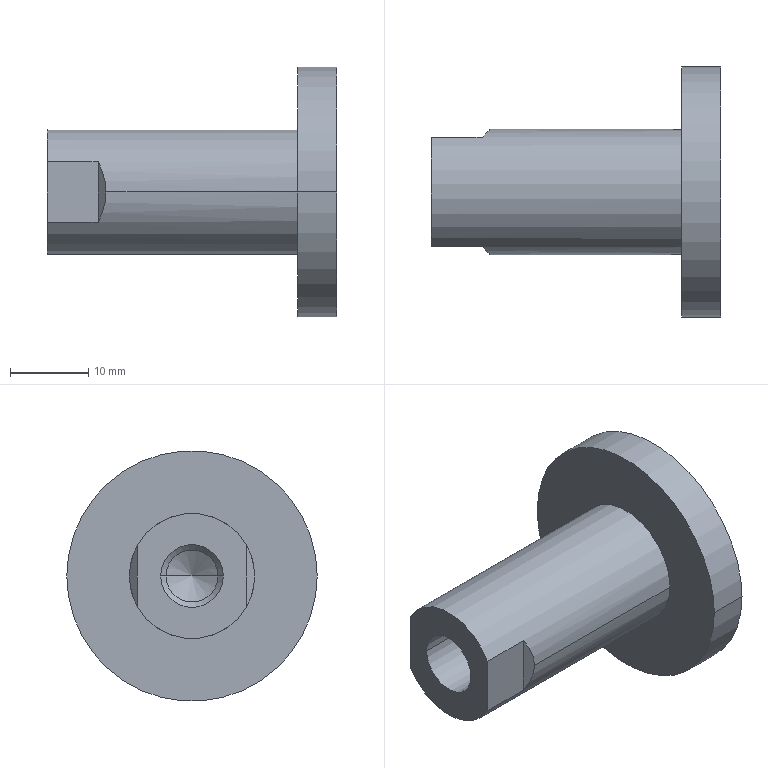Part | STEP file | [儘僢僪]-4 | 1 solid | 19 faces | box 37 x 32 x 32 mm | volume 9768 mm3 | cylinder 8 | plane 7 | cone 4 | commonest cylinder face diameters 6.647 x2 8 x2 16 x2 32 x2
STEP:
#1=CARTESIAN_POINT('',(0.,0.,0.));
#2=DIRECTION('',(0.,0.,1.));
#3=DIRECTION('',(1.,0.,0.));
#4=AXIS2_PLACEMENT_3D('',#1,#2,#3);
#5=CARTESIAN_POINT('',(4.426,25.824,22.5));
#6=VERTEX_POINT('',#5);
#7=CARTESIAN_POINT('',(8.,25.823,22.5));
#8=VERTEX_POINT('',#7);
#9=CARTESIAN_POINT('',(32.,25.823,22.5));
#10=DIRECTION('',(1.,0.,0.));
#11=VECTOR('',#10,1.);
#12=LINE('',#9,#11);
#13=CARTESIAN_POINT('',(32.,22.5,22.5));
#14=DIRECTION('',(1.,0.,0.));
#15=DIRECTION('',(0.,1.,0.));
#16=AXIS2_PLACEMENT_3D('',#13,#14,#15);
#17=CYLINDRICAL_SURFACE('',#16,3.324);
#18=CARTESIAN_POINT('',(6.283,0.));
#19=DIRECTION('',(0.,1.));
#20=VECTOR('',#19,1.);
#21=LINE('',#18,#20);
#22=(GEOMETRIC_REPRESENTATION_CONTEXT(2)PARAMETRIC_REPRESENTATION_CONTEXT()REPRESENTATION_CONTEXT('',''));
#23=DEFINITIONAL_REPRESENTATION('',(#21),#22);
#24=PCURVE('',#17,#23);
#25=CARTESIAN_POINT('',(32.,22.5,22.5));
#26=DIRECTION('',(1.,0.,0.));
#27=DIRECTION('',(0.,1.,0.));
#28=AXIS2_PLACEMENT_3D('',#25,#26,#27);
#29=CYLINDRICAL_SURFACE('',#28,3.324);
#30=CARTESIAN_POINT('',(0.,0.));
#31=DIRECTION('',(0.,1.));
#32=VECTOR('',#31,1.);
#33=LINE('',#30,#32);
#34=(GEOMETRIC_REPRESENTATION_CONTEXT(2)PARAMETRIC_REPRESENTATION_CONTEXT()REPRESENTATION_CONTEXT('',''));
#35=DEFINITIONAL_REPRESENTATION('',(#33),#34);
#36=PCURVE('',#29,#35);
#37=SURFACE_CURVE('',#12,(#24,#36),.PCURVE_S1.);
#38=EDGE_CURVE('',#6,#8,#37,.T.);
#39=ORIENTED_EDGE('',*,*,#38,.T.);
#40=CARTESIAN_POINT('',(8.,19.177,22.5));
#41=VERTEX_POINT('',#40);
#42=CARTESIAN_POINT('',(8.,22.5,22.5));
#43=DIRECTION('',(1.,0.,0.));
#44=DIRECTION('',(0.,1.,0.));
#45=AXIS2_PLACEMENT_3D('',#42,#43,#44);
#46=CIRCLE('',#45,3.324);
#47=CARTESIAN_POINT('',(0.,-24.));
#48=DIRECTION('',(1.,0.));
#49=VECTOR('',#48,1.);
#50=LINE('',#47,#49);
#51=(GEOMETRIC_REPRESENTATION_CONTEXT(2)PARAMETRIC_REPRESENTATION_CONTEXT()REPRESENTATION_CONTEXT('',''));
#52=DEFINITIONAL_REPRESENTATION('',(#50),#51);
#53=PCURVE('',#17,#52);
#54=CARTESIAN_POINT('',(-990.081,22.5,22.5));
#55=DIRECTION('',(-1.,0.,0.));
#56=DIRECTION('',(0.,-1.,0.));
#57=AXIS2_PLACEMENT_3D('',#54,#55,#56);
#58=CONICAL_SURFACE('',#57,1732.051,1.047);
#59=CARTESIAN_POINT('',(9.425,-998.081));
#60=DIRECTION('',(-1.,0.));
#61=VECTOR('',#60,1.);
#62=LINE('',#59,#61);
#63=(GEOMETRIC_REPRESENTATION_CONTEXT(2)PARAMETRIC_REPRESENTATION_CONTEXT()REPRESENTATION_CONTEXT('',''));
#64=DEFINITIONAL_REPRESENTATION('',(#62),#63);
#65=PCURVE('',#58,#64);
#66=SURFACE_CURVE('',#46,(#53,#65),.PCURVE_S1.);
#67=EDGE_CURVE('',#41,#8,#66,.T.);
#68=ORIENTED_EDGE('',*,*,#67,.F.);
#69=CARTESIAN_POINT('',(4.426,19.177,22.5));
#70=VERTEX_POINT('',#69);
#71=CARTESIAN_POINT('',(32.,19.177,22.5));
#72=DIRECTION('',(1.,0.,0.));
#73=VECTOR('',#72,1.);
#74=LINE('',#71,#73);
#75=CARTESIAN_POINT('',(3.142,0.));
#76=DIRECTION('',(0.,1.));
#77=VECTOR('',#76,1.);
#78=LINE('',#75,#77);
#79=(GEOMETRIC_REPRESENTATION_CONTEXT(2)PARAMETRIC_REPRESENTATION_CONTEXT()REPRESENTATION_CONTEXT('',''));
#80=DEFINITIONAL_REPRESENTATION('',(#78),#79);
#81=PCURVE('',#17,#80);
#82=CARTESIAN_POINT('',(3.142,0.));
#83=DIRECTION('',(0.,1.));
#84=VECTOR('',#83,1.);
#85=LINE('',#82,#84);
#86=(GEOMETRIC_REPRESENTATION_CONTEXT(2)PARAMETRIC_REPRESENTATION_CONTEXT()REPRESENTATION_CONTEXT('',''));
#87=DEFINITIONAL_REPRESENTATION('',(#85),#86);
#88=PCURVE('',#29,#87);
#89=SURFACE_CURVE('',#74,(#81,#88),.PCURVE_S1.);
#90=EDGE_CURVE('',#70,#41,#89,.T.);
#91=ORIENTED_EDGE('',*,*,#90,.F.);
#92=CARTESIAN_POINT('',(4.426,22.5,22.5));
#93=DIRECTION('',(1.,0.,0.));
#94=DIRECTION('',(0.,-1.,0.));
#95=AXIS2_PLACEMENT_3D('',#92,#93,#94);
#96=CIRCLE('',#95,3.324);
#97=CARTESIAN_POINT('',(3.142,-27.573));
#98=DIRECTION('',(1.,0.));
#99=VECTOR('',#98,1.);
#100=LINE('',#97,#99);
#101=(GEOMETRIC_REPRESENTATION_CONTEXT(2)PARAMETRIC_REPRESENTATION_CONTEXT()REPRESENTATION_CONTEXT('',''));
#102=DEFINITIONAL_REPRESENTATION('',(#100),#101);
#103=PCURVE('',#17,#102);
#104=CARTESIAN_POINT('',(5.,22.5,22.5));
#105=DIRECTION('',(-1.,0.,0.));
#106=DIRECTION('',(0.,-1.,0.));
#107=AXIS2_PLACEMENT_3D('',#104,#105,#106);
#108=CONICAL_SURFACE('',#107,2.75,0.7854);
#109=CARTESIAN_POINT('',(6.283,0.5735));
#110=DIRECTION('',(-1.,0.));
#111=VECTOR('',#110,1.);
#112=LINE('',#109,#111);
#113=(GEOMETRIC_REPRESENTATION_CONTEXT(2)PARAMETRIC_REPRESENTATION_CONTEXT()REPRESENTATION_CONTEXT('',''));
#114=DEFINITIONAL_REPRESENTATION('',(#112),#113);
#115=PCURVE('',#108,#114);
#116=SURFACE_CURVE('',#96,(#103,#115),.PCURVE_S1.);
#117=EDGE_CURVE('',#70,#6,#116,.T.);
#118=ORIENTED_EDGE('',*,*,#117,.T.);
#119=EDGE_LOOP('',(#39,#68,#91,#118));
#120=FACE_BOUND('',#119,.F.);
#121=ADVANCED_FACE('',(#120),#17,.F.);
#122=ORIENTED_EDGE('',*,*,#67,.T.);
#123=CARTESIAN_POINT('',(9.919,22.5,22.5));
#124=VERTEX_POINT('',#123);
#125=CARTESIAN_POINT('',(9.919,22.5,22.5));
#126=DIRECTION('',(-0.5,0.866,0.));
#127=VECTOR('',#126,1.);
#128=LINE('',#125,#127);
#129=CARTESIAN_POINT('',(3.142,-1000.));
#130=CARTESIAN_POINT('',(3.142,-999.971));
#131=CARTESIAN_POINT('',(3.142,-999.913));
#132=CARTESIAN_POINT('',(3.142,-999.826));
#133=CARTESIAN_POINT('',(3.142,-999.738));
#134=CARTESIAN_POINT('',(3.142,-999.651));
#135=CARTESIAN_POINT('',(3.142,-999.564));
#136=CARTESIAN_POINT('',(3.142,-999.477));
#137=CARTESIAN_POINT('',(3.142,-999.389));
#138=CARTESIAN_POINT('',(3.142,-999.302));
#139=CARTESIAN_POINT('',(3.142,-999.215));
#140=CARTESIAN_POINT('',(3.142,-999.128));
#141=CARTESIAN_POINT('',(3.142,-999.041));
#142=CARTESIAN_POINT('',(3.142,-998.953));
#143=CARTESIAN_POINT('',(3.142,-998.866));
#144=CARTESIAN_POINT('',(3.142,-998.779));
#145=CARTESIAN_POINT('',(3.142,-998.692));
#146=CARTESIAN_POINT('',(3.142,-998.604));
#147=CARTESIAN_POINT('',(3.142,-998.517));
#148=CARTESIAN_POINT('',(3.142,-998.43));
#149=CARTESIAN_POINT('',(3.142,-998.343));
#150=CARTESIAN_POINT('',(3.142,-998.256));
#151=CARTESIAN_POINT('',(3.142,-998.168));
#152=CARTESIAN_POINT('',(3.142,-998.11));
#153=CARTESIAN_POINT('',(3.142,-998.081));
#154=B_SPLINE_CURVE_WITH_KNOTS('',3,(#129,#130,#131,#132,#133,#134,#135,#136,#137,#138,#139,#140,#141,#142,#143,#144,#145,#146,#147,#148,#149,#150,#151,#152,#153),.UNSPECIFIED.,.F.,.F.,(4,1,1,1,1,1,1,1,1,1,1,1,1,1,1,1,1,1,1,1,1,1,4),(0.,0.1744,0.3489,0.5233,0.6978,0.8722,1.047,1.221,1.396,1.57,1.744,1.919,2.093,2.268,2.442,2.617,2.791,2.965,3.14,3.314,3.489,3.663,3.838),.QUASI_UNIFORM_KNOTS.);
#155=(GEOMETRIC_REPRESENTATION_CONTEXT(2)PARAMETRIC_REPRESENTATION_CONTEXT()REPRESENTATION_CONTEXT('',''));
#156=DEFINITIONAL_REPRESENTATION('',(#154),#155);
#157=PCURVE('',#58,#156);
#158=CARTESIAN_POINT('',(-990.081,22.5,22.5));
#159=DIRECTION('',(-1.,0.,0.));
#160=DIRECTION('',(0.,-1.,0.));
#161=AXIS2_PLACEMENT_3D('',#158,#159,#160);
#162=CONICAL_SURFACE('',#161,1732.051,1.047);
#163=CARTESIAN_POINT('',(3.142,-1000.));
#164=CARTESIAN_POINT('',(3.142,-999.971));
#165=CARTESIAN_POINT('',(3.142,-999.913));
#166=CARTESIAN_POINT('',(3.142,-999.826));
#167=CARTESIAN_POINT('',(3.142,-999.738));
#168=CARTESIAN_POINT('',(3.142,-999.651));
#169=CARTESIAN_POINT('',(3.142,-999.564));
#170=CARTESIAN_POINT('',(3.142,-999.477));
#171=CARTESIAN_POINT('',(3.142,-999.389));
#172=CARTESIAN_POINT('',(3.142,-999.302));
#173=CARTESIAN_POINT('',(3.142,-999.215));
#174=CARTESIAN_POINT('',(3.142,-999.128));
#175=CARTESIAN_POINT('',(3.142,-999.041));
#176=CARTESIAN_POINT('',(3.142,-998.953));
#177=CARTESIAN_POINT('',(3.142,-998.866));
#178=CARTESIAN_POINT('',(3.142,-998.779));
#179=CARTESIAN_POINT('',(3.142,-998.692));
#180=CARTESIAN_POINT('',(3.142,-998.604));
#181=CARTESIAN_POINT('',(3.142,-998.517));
#182=CARTESIAN_POINT('',(3.142,-998.43));
#183=CARTESIAN_POINT('',(3.142,-998.343));
#184=CARTESIAN_POINT('',(3.142,-998.256));
#185=CARTESIAN_POINT('',(3.142,-998.168));
#186=CARTESIAN_POINT('',(3.142,-998.11));
#187=CARTESIAN_POINT('',(3.142,-998.081));
#188=B_SPLINE_CURVE_WITH_KNOTS('',3,(#163,#164,#165,#166,#167,#168,#169,#170,#171,#172,#173,#174,#175,#176,#177,#178,#179,#180,#181,#182,#183,#184,#185,#186,#187),.UNSPECIFIED.,.F.,.F.,(4,1,1,1,1,1,1,1,1,1,1,1,1,1,1,1,1,1,1,1,1,1,4),(0.,0.1744,0.3489,0.5233,0.6978,0.8722,1.047,1.221,1.396,1.57,1.744,1.919,2.093,2.268,2.442,2.617,2.791,2.965,3.14,3.314,3.489,3.663,3.838),.QUASI_UNIFORM_KNOTS.);
#189=(GEOMETRIC_REPRESENTATION_CONTEXT(2)PARAMETRIC_REPRESENTATION_CONTEXT()REPRESENTATION_CONTEXT('',''));
#190=DEFINITIONAL_REPRESENTATION('',(#188),#189);
#191=PCURVE('',#162,#190);
#192=SURFACE_CURVE('',#128,(#157,#191),.PCURVE_S1.);
#193=EDGE_CURVE('',#124,#8,#192,.T.);
#194=ORIENTED_EDGE('',*,*,#193,.F.);
#195=CARTESIAN_POINT('',(9.919,22.5,22.5));
#196=DIRECTION('',(-0.5,-0.866,0.));
#197=VECTOR('',#196,1.);
#198=LINE('',#195,#197);
#199=CARTESIAN_POINT('',(6.283,-1000.));
#200=DIRECTION('',(0.,1.));
#201=VECTOR('',#200,1.);
#202=LINE('',#199,#201);
#203=(GEOMETRIC_REPRESENTATION_CONTEXT(2)PARAMETRIC_REPRESENTATION_CONTEXT()REPRESENTATION_CONTEXT('',''));
#204=DEFINITIONAL_REPRESENTATION('',(#202),#203);
#205=PCURVE('',#58,#204);
#206=CARTESIAN_POINT('',(0.,-1000.));
#207=DIRECTION('',(0.,1.));
#208=VECTOR('',#207,1.);
#209=LINE('',#206,#208);
#210=(GEOMETRIC_REPRESENTATION_CONTEXT(2)PARAMETRIC_REPRESENTATION_CONTEXT()REPRESENTATION_CONTEXT('',''));
#211=DEFINITIONAL_REPRESENTATION('',(#209),#210);
#212=PCURVE('',#162,#211);
#213=SURFACE_CURVE('',#198,(#205,#212),.PCURVE_S1.);
#214=EDGE_CURVE('',#124,#41,#213,.T.);
#215=ORIENTED_EDGE('',*,*,#214,.T.);
#216=EDGE_LOOP('',(#122,#194,#215));
#217=FACE_BOUND('',#216,.F.);
#218=ADVANCED_FACE('',(#217),#58,.F.);
#219=CARTESIAN_POINT('',(3.75,18.5,22.5));
#220=VERTEX_POINT('',#219);
#221=CARTESIAN_POINT('',(-5.,18.5,22.5));
#222=VERTEX_POINT('',#221);
#223=CARTESIAN_POINT('',(-32.,18.5,22.5));
#224=DIRECTION('',(-1.,0.,0.));
#225=VECTOR('',#224,1.);
#226=LINE('',#223,#225);
#227=CARTESIAN_POINT('',(-32.,22.5,22.5));
#228=DIRECTION('',(-1.,0.,0.));
#229=DIRECTION('',(0.,-1.,0.));
#230=AXIS2_PLACEMENT_3D('',#227,#228,#229);
#231=CYLINDRICAL_SURFACE('',#230,4.);
#232=CARTESIAN_POINT('',(6.283,0.));
#233=DIRECTION('',(0.,1.));
#234=VECTOR('',#233,1.);
#235=LINE('',#232,#234);
#236=(GEOMETRIC_REPRESENTATION_CONTEXT(2)PARAMETRIC_REPRESENTATION_CONTEXT()REPRESENTATION_CONTEXT('',''));
#237=DEFINITIONAL_REPRESENTATION('',(#235),#236);
#238=PCURVE('',#231,#237);
#239=CARTESIAN_POINT('',(-32.,22.5,22.5));
#240=DIRECTION('',(-1.,0.,0.));
#241=DIRECTION('',(0.,-1.,0.));
#242=AXIS2_PLACEMENT_3D('',#239,#240,#241);
#243=CYLINDRICAL_SURFACE('',#242,4.);
#244=CARTESIAN_POINT('',(0.,0.));
#245=DIRECTION('',(0.,1.));
#246=VECTOR('',#245,1.);
#247=LINE('',#244,#246);
#248=(GEOMETRIC_REPRESENTATION_CONTEXT(2)PARAMETRIC_REPRESENTATION_CONTEXT()REPRESENTATION_CONTEXT('',''));
#249=DEFINITIONAL_REPRESENTATION('',(#247),#248);
#250=PCURVE('',#243,#249);
#251=SURFACE_CURVE('',#226,(#238,#250),.PCURVE_S1.);
#252=EDGE_CURVE('',#220,#222,#251,.T.);
#253=ORIENTED_EDGE('',*,*,#252,.T.);
#254=CARTESIAN_POINT('',(-5.,26.5,22.5));
#255=VERTEX_POINT('',#254);
#256=CARTESIAN_POINT('',(-5.,22.5,22.5));
#257=DIRECTION('',(-1.,0.,0.));
#258=DIRECTION('',(0.,-1.,0.));
#259=AXIS2_PLACEMENT_3D('',#256,#257,#258);
#260=CIRCLE('',#259,4.);
#261=CARTESIAN_POINT('',(0.,-27.));
#262=DIRECTION('',(1.,0.));
#263=VECTOR('',#262,1.);
#264=LINE('',#261,#263);
#265=(GEOMETRIC_REPRESENTATION_CONTEXT(2)PARAMETRIC_REPRESENTATION_CONTEXT()REPRESENTATION_CONTEXT('',''));
#266=DEFINITIONAL_REPRESENTATION('',(#264),#265);
#267=PCURVE('',#231,#266);
#268=CARTESIAN_POINT('',(-5.,22.5,26.5));
#269=DIRECTION('',(1.,0.,0.));
#270=DIRECTION('',(0.,1.,0.));
#271=AXIS2_PLACEMENT_3D('',#268,#269,#270);
#272=PLANE('',#271);
#273=CARTESIAN_POINT('',(-4.,-4.));
#274=CARTESIAN_POINT('',(-4.,2.928));
#275=CARTESIAN_POINT('',(2.,-0.5359));
#276=CARTESIAN_POINT('',(8.,-4.));
#277=CARTESIAN_POINT('',(2.,-7.464));
#278=CARTESIAN_POINT('',(-4.,-10.928));
#279=CARTESIAN_POINT('',(-4.,-4.));
#280=(BOUNDED_CURVE()B_SPLINE_CURVE(2,(#273,#274,#275,#276,#277,#278,#279),.UNSPECIFIED.,.T.,.F.)B_SPLINE_CURVE_WITH_KNOTS((1,2,2,2,2,1),(-2.094,0.,2.094,4.189,6.283,8.378),.UNSPECIFIED.)CURVE()GEOMETRIC_REPRESENTATION_ITEM()RATIONAL_B_SPLINE_CURVE((1.,0.5,1.,0.5,1.,0.5,1.))REPRESENTATION_ITEM(''));
#281=(GEOMETRIC_REPRESENTATION_CONTEXT(2)PARAMETRIC_REPRESENTATION_CONTEXT()REPRESENTATION_CONTEXT('',''));
#282=DEFINITIONAL_REPRESENTATION('',(#280),#281);
#283=PCURVE('',#272,#282);
#284=SURFACE_CURVE('',#260,(#267,#283),.PCURVE_S1.);
#285=EDGE_CURVE('',#255,#222,#284,.T.);
#286=ORIENTED_EDGE('',*,*,#285,.F.);
#287=CARTESIAN_POINT('',(3.75,26.5,22.5));
#288=VERTEX_POINT('',#287);
#289=CARTESIAN_POINT('',(-32.,26.5,22.5));
#290=DIRECTION('',(-1.,0.,0.));
#291=VECTOR('',#290,1.);
#292=LINE('',#289,#291);
#293=CARTESIAN_POINT('',(3.142,0.));
#294=DIRECTION('',(0.,1.));
#295=VECTOR('',#294,1.);
#296=LINE('',#293,#295);
#297=(GEOMETRIC_REPRESENTATION_CONTEXT(2)PARAMETRIC_REPRESENTATION_CONTEXT()REPRESENTATION_CONTEXT('',''));
#298=DEFINITIONAL_REPRESENTATION('',(#296),#297);
#299=PCURVE('',#231,#298);
#300=CARTESIAN_POINT('',(3.142,0.));
#301=DIRECTION('',(0.,1.));
#302=VECTOR('',#301,1.);
#303=LINE('',#300,#302);
#304=(GEOMETRIC_REPRESENTATION_CONTEXT(2)PARAMETRIC_REPRESENTATION_CONTEXT()REPRESENTATION_CONTEXT('',''));
#305=DEFINITIONAL_REPRESENTATION('',(#303),#304);
#306=PCURVE('',#243,#305);
#307=SURFACE_CURVE('',#292,(#299,#306),.PCURVE_S1.);
#308=EDGE_CURVE('',#288,#255,#307,.T.);
#309=ORIENTED_EDGE('',*,*,#308,.F.);
#310=CARTESIAN_POINT('',(3.75,22.5,22.5));
#311=DIRECTION('',(-1.,0.,0.));
#312=DIRECTION('',(0.,-1.,0.));
#313=AXIS2_PLACEMENT_3D('',#310,#311,#312);
#314=CIRCLE('',#313,4.);
#315=CARTESIAN_POINT('',(0.,-35.75));
#316=DIRECTION('',(1.,0.));
#317=VECTOR('',#316,1.);
#318=LINE('',#315,#317);
#319=(GEOMETRIC_REPRESENTATION_CONTEXT(2)PARAMETRIC_REPRESENTATION_CONTEXT()REPRESENTATION_CONTEXT('',''));
#320=DEFINITIONAL_REPRESENTATION('',(#318),#319);
#321=PCURVE('',#231,#320);
#322=CARTESIAN_POINT('',(0.,1.25));
#323=DIRECTION('',(1.,0.));
#324=VECTOR('',#323,1.);
#325=LINE('',#322,#324);
#326=(GEOMETRIC_REPRESENTATION_CONTEXT(2)PARAMETRIC_REPRESENTATION_CONTEXT()REPRESENTATION_CONTEXT('',''));
#327=DEFINITIONAL_REPRESENTATION('',(#325),#326);
#328=PCURVE('',#108,#327);
#329=SURFACE_CURVE('',#314,(#321,#328),.PCURVE_S1.);
#330=EDGE_CURVE('',#288,#220,#329,.T.);
#331=ORIENTED_EDGE('',*,*,#330,.T.);
#332=EDGE_LOOP('',(#253,#286,#309,#331));
#333=FACE_BOUND('',#332,.F.);
#334=ADVANCED_FACE('',(#333),#231,.F.);
#335=CARTESIAN_POINT('',(5.,19.75,22.5));
#336=DIRECTION('',(-0.7071,-0.7071,0.));
#337=VECTOR('',#336,1.);
#338=LINE('',#335,#337);
#339=CARTESIAN_POINT('',(6.283,0.));
#340=DIRECTION('',(0.,1.));
#341=VECTOR('',#340,1.);
#342=LINE('',#339,#341);
#343=(GEOMETRIC_REPRESENTATION_CONTEXT(2)PARAMETRIC_REPRESENTATION_CONTEXT()REPRESENTATION_CONTEXT('',''));
#344=DEFINITIONAL_REPRESENTATION('',(#342),#343);
#345=PCURVE('',#108,#344);
#346=CARTESIAN_POINT('',(5.,22.5,22.5));
#347=DIRECTION('',(-1.,0.,0.));
#348=DIRECTION('',(0.,-1.,0.));
#349=AXIS2_PLACEMENT_3D('',#346,#347,#348);
#350=CONICAL_SURFACE('',#349,2.75,0.7854);
#351=CARTESIAN_POINT('',(0.,0.));
#352=DIRECTION('',(0.,1.));
#353=VECTOR('',#352,1.);
#354=LINE('',#351,#353);
#355=(GEOMETRIC_REPRESENTATION_CONTEXT(2)PARAMETRIC_REPRESENTATION_CONTEXT()REPRESENTATION_CONTEXT('',''));
#356=DEFINITIONAL_REPRESENTATION('',(#354),#355);
#357=PCURVE('',#350,#356);
#358=SURFACE_CURVE('',#338,(#345,#357),.PCURVE_S1.);
#359=EDGE_CURVE('',#70,#220,#358,.T.);
#360=ORIENTED_EDGE('',*,*,#359,.T.);
#361=ORIENTED_EDGE('',*,*,#330,.F.);
#362=CARTESIAN_POINT('',(5.,25.25,22.5));
#363=DIRECTION('',(-0.7071,0.7071,0.));
#364=VECTOR('',#363,1.);
#365=LINE('',#362,#364);
#366=CARTESIAN_POINT('',(3.142,0.));
#367=DIRECTION('',(0.,1.));
#368=VECTOR('',#367,1.);
#369=LINE('',#366,#368);
#370=(GEOMETRIC_REPRESENTATION_CONTEXT(2)PARAMETRIC_REPRESENTATION_CONTEXT()REPRESENTATION_CONTEXT('',''));
#371=DEFINITIONAL_REPRESENTATION('',(#369),#370);
#372=PCURVE('',#108,#371);
#373=CARTESIAN_POINT('',(3.142,0.));
#374=DIRECTION('',(0.,1.));
#375=VECTOR('',#374,1.);
#376=LINE('',#373,#375);
#377=(GEOMETRIC_REPRESENTATION_CONTEXT(2)PARAMETRIC_REPRESENTATION_CONTEXT()REPRESENTATION_CONTEXT('',''));
#378=DEFINITIONAL_REPRESENTATION('',(#376),#377);
#379=PCURVE('',#350,#378);
#380=SURFACE_CURVE('',#365,(#372,#379),.PCURVE_S1.);
#381=EDGE_CURVE('',#6,#288,#380,.T.);
#382=ORIENTED_EDGE('',*,*,#381,.F.);
#383=ORIENTED_EDGE('',*,*,#117,.F.);
#384=EDGE_LOOP('',(#360,#361,#382,#383));
#385=FACE_BOUND('',#384,.F.);
#386=ADVANCED_FACE('',(#385),#108,.F.);
#387=CARTESIAN_POINT('',(27.,38.5,22.5));
#388=VERTEX_POINT('',#387);
#389=CARTESIAN_POINT('',(27.,6.5,22.5));
#390=VERTEX_POINT('',#389);
#391=CARTESIAN_POINT('',(27.,22.5,22.5));
#392=DIRECTION('',(1.,0.,0.));
#393=DIRECTION('',(0.,1.,0.));
#394=AXIS2_PLACEMENT_3D('',#391,#392,#393);
#395=CIRCLE('',#394,16.);
#396=CARTESIAN_POINT('',(32.,22.5,22.5));
#397=DIRECTION('',(1.,0.,0.));
#398=DIRECTION('',(0.,1.,0.));
#399=AXIS2_PLACEMENT_3D('',#396,#397,#398);
#400=CYLINDRICAL_SURFACE('',#399,16.);
#401=CARTESIAN_POINT('',(0.,-5.));
#402=DIRECTION('',(1.,0.));
#403=VECTOR('',#402,1.);
#404=LINE('',#401,#403);
#405=(GEOMETRIC_REPRESENTATION_CONTEXT(2)PARAMETRIC_REPRESENTATION_CONTEXT()REPRESENTATION_CONTEXT('',''));
#406=DEFINITIONAL_REPRESENTATION('',(#404),#405);
#407=PCURVE('',#400,#406);
#408=CARTESIAN_POINT('',(27.,22.5,30.5));
#409=DIRECTION('',(1.,0.,0.));
#410=DIRECTION('',(0.,1.,0.));
#411=AXIS2_PLACEMENT_3D('',#408,#409,#410);
#412=PLANE('',#411);
#413=CARTESIAN_POINT('',(0.,-8.));
#414=DIRECTION('',(1.,0.));
#415=AXIS2_PLACEMENT_2D('',#413,#414);
#416=CIRCLE('',#415,16.);
#417=(GEOMETRIC_REPRESENTATION_CONTEXT(2)PARAMETRIC_REPRESENTATION_CONTEXT()REPRESENTATION_CONTEXT('',''));
#418=DEFINITIONAL_REPRESENTATION('',(#416),#417);
#419=PCURVE('',#412,#418);
#420=SURFACE_CURVE('',#395,(#407,#419),.PCURVE_S1.);
#421=EDGE_CURVE('',#388,#390,#420,.T.);
#422=ORIENTED_EDGE('',*,*,#421,.T.);
#423=CARTESIAN_POINT('',(32.,6.5,22.5));
#424=VERTEX_POINT('',#423);
#425=CARTESIAN_POINT('',(32.,6.5,22.5));
#426=DIRECTION('',(1.,0.,0.));
#427=VECTOR('',#426,1.);
#428=LINE('',#425,#427);
#429=CARTESIAN_POINT('',(3.142,0.));
#430=DIRECTION('',(0.,1.));
#431=VECTOR('',#430,1.);
#432=LINE('',#429,#431);
#433=(GEOMETRIC_REPRESENTATION_CONTEXT(2)PARAMETRIC_REPRESENTATION_CONTEXT()REPRESENTATION_CONTEXT('',''));
#434=DEFINITIONAL_REPRESENTATION('',(#432),#433);
#435=PCURVE('',#400,#434);
#436=CARTESIAN_POINT('',(32.,22.5,22.5));
#437=DIRECTION('',(1.,0.,0.));
#438=DIRECTION('',(0.,1.,0.));
#439=AXIS2_PLACEMENT_3D('',#436,#437,#438);
#440=CYLINDRICAL_SURFACE('',#439,16.);
#441=CARTESIAN_POINT('',(3.142,0.));
#442=DIRECTION('',(0.,1.));
#443=VECTOR('',#442,1.);
#444=LINE('',#441,#443);
#445=(GEOMETRIC_REPRESENTATION_CONTEXT(2)PARAMETRIC_REPRESENTATION_CONTEXT()REPRESENTATION_CONTEXT('',''));
#446=DEFINITIONAL_REPRESENTATION('',(#444),#445);
#447=PCURVE('',#440,#446);
#448=SURFACE_CURVE('',#428,(#435,#447),.PCURVE_S1.);
#449=EDGE_CURVE('',#390,#424,#448,.T.);
#450=ORIENTED_EDGE('',*,*,#449,.T.);
#451=CARTESIAN_POINT('',(32.,38.5,22.5));
#452=VERTEX_POINT('',#451);
#453=CARTESIAN_POINT('',(32.,22.5,22.5));
#454=DIRECTION('',(1.,0.,0.));
#455=DIRECTION('',(0.,1.,0.));
#456=AXIS2_PLACEMENT_3D('',#453,#454,#455);
#457=CIRCLE('',#456,16.);
#458=CARTESIAN_POINT('',(0.,0.));
#459=DIRECTION('',(1.,0.));
#460=VECTOR('',#459,1.);
#461=LINE('',#458,#460);
#462=(GEOMETRIC_REPRESENTATION_CONTEXT(2)PARAMETRIC_REPRESENTATION_CONTEXT()REPRESENTATION_CONTEXT('',''));
#463=DEFINITIONAL_REPRESENTATION('',(#461),#462);
#464=PCURVE('',#400,#463);
#465=CARTESIAN_POINT('',(32.,22.5,38.5));
#466=DIRECTION('',(-1.,0.,0.));
#467=DIRECTION('',(0.,-1.,0.));
#468=AXIS2_PLACEMENT_3D('',#465,#466,#467);
#469=PLANE('',#468);
#470=CARTESIAN_POINT('',(-16.,-16.));
#471=CARTESIAN_POINT('',(-16.,11.713));
#472=CARTESIAN_POINT('',(8.,-2.144));
#473=CARTESIAN_POINT('',(32.,-16.));
#474=CARTESIAN_POINT('',(8.,-29.856));
#475=CARTESIAN_POINT('',(-16.,-43.713));
#476=CARTESIAN_POINT('',(-16.,-16.));
#477=(BOUNDED_CURVE()B_SPLINE_CURVE(2,(#470,#471,#472,#473,#474,#475,#476),.UNSPECIFIED.,.T.,.F.)B_SPLINE_CURVE_WITH_KNOTS((1,2,2,2,2,1),(-2.094,0.,2.094,4.189,6.283,8.378),.UNSPECIFIED.)CURVE()GEOMETRIC_REPRESENTATION_ITEM()RATIONAL_B_SPLINE_CURVE((1.,0.5,1.,0.5,1.,0.5,1.))REPRESENTATION_ITEM(''));
#478=(GEOMETRIC_REPRESENTATION_CONTEXT(2)PARAMETRIC_REPRESENTATION_CONTEXT()REPRESENTATION_CONTEXT('',''));
#479=DEFINITIONAL_REPRESENTATION('',(#477),#478);
#480=PCURVE('',#469,#479);
#481=SURFACE_CURVE('',#457,(#464,#480),.PCURVE_S1.);
#482=EDGE_CURVE('',#452,#424,#481,.T.);
#483=ORIENTED_EDGE('',*,*,#482,.F.);
#484=CARTESIAN_POINT('',(32.,38.5,22.5));
#485=DIRECTION('',(1.,0.,0.));
#486=VECTOR('',#485,1.);
#487=LINE('',#484,#486);
#488=CARTESIAN_POINT('',(0.,0.));
#489=DIRECTION('',(0.,1.));
#490=VECTOR('',#489,1.);
#491=LINE('',#488,#490);
#492=(GEOMETRIC_REPRESENTATION_CONTEXT(2)PARAMETRIC_REPRESENTATION_CONTEXT()REPRESENTATION_CONTEXT('',''));
#493=DEFINITIONAL_REPRESENTATION('',(#491),#492);
#494=PCURVE('',#400,#493);
#495=CARTESIAN_POINT('',(6.283,0.));
#496=DIRECTION('',(0.,1.));
#497=VECTOR('',#496,1.);
#498=LINE('',#495,#497);
#499=(GEOMETRIC_REPRESENTATION_CONTEXT(2)PARAMETRIC_REPRESENTATION_CONTEXT()REPRESENTATION_CONTEXT('',''));
#500=DEFINITIONAL_REPRESENTATION('',(#498),#499);
#501=PCURVE('',#440,#500);
#502=SURFACE_CURVE('',#487,(#494,#501),.PCURVE_S1.);
#503=EDGE_CURVE('',#388,#452,#502,.T.);
#504=ORIENTED_EDGE('',*,*,#503,.F.);
#505=EDGE_LOOP('',(#422,#450,#483,#504));
#506=FACE_BOUND('',#505,.T.);
#507=ADVANCED_FACE('',(#506),#400,.T.);
#508=CARTESIAN_POINT('',(2.5,14.5,22.5));
#509=VERTEX_POINT('',#508);
#510=CARTESIAN_POINT('',(1.5,15.5,26.373));
#511=VERTEX_POINT('',#510);
#512=CARTESIAN_POINT('',(2.5,14.5,22.5));
#513=CARTESIAN_POINT('',(2.5,14.5,23.862));
#514=CARTESIAN_POINT('',(2.159,14.841,25.181));
#515=CARTESIAN_POINT('',(1.5,15.5,26.373));
#516=(BOUNDED_CURVE()B_SPLINE_CURVE(3,(#512,#513,#514,#515),.UNSPECIFIED.,.F.,.F.)B_SPLINE_CURVE_WITH_KNOTS((4,4),(0.,0.5054),.PIECEWISE_BEZIER_KNOTS.)CURVE()GEOMETRIC_REPRESENTATION_ITEM()RATIONAL_B_SPLINE_CURVE((1.,0.9788,0.9788,1.))REPRESENTATION_ITEM(''));
#517=CARTESIAN_POINT('',(32.,22.5,22.5));
#518=DIRECTION('',(1.,0.,0.));
#519=DIRECTION('',(0.,1.,0.));
#520=AXIS2_PLACEMENT_3D('',#517,#518,#519);
#521=CYLINDRICAL_SURFACE('',#520,8.);
#522=CARTESIAN_POINT('',(3.142,-29.5));
#523=CARTESIAN_POINT('',(3.134,-29.5));
#524=CARTESIAN_POINT('',(3.119,-29.501));
#525=CARTESIAN_POINT('',(3.096,-29.508));
#526=CARTESIAN_POINT('',(3.073,-29.518));
#527=CARTESIAN_POINT('',(3.05,-29.533));
#528=CARTESIAN_POINT('',(3.027,-29.552));
#529=CARTESIAN_POINT('',(3.004,-29.575));
#530=CARTESIAN_POINT('',(2.981,-29.602));
#531=CARTESIAN_POINT('',(2.958,-29.634));
#532=CARTESIAN_POINT('',(2.935,-29.669));
#533=CARTESIAN_POINT('',(2.912,-29.709));
#534=CARTESIAN_POINT('',(2.889,-29.753));
#535=CARTESIAN_POINT('',(2.866,-29.802));
#536=CARTESIAN_POINT('',(2.843,-29.854));
#537=CARTESIAN_POINT('',(2.82,-29.91));
#538=CARTESIAN_POINT('',(2.797,-29.971));
#539=CARTESIAN_POINT('',(2.774,-30.035));
#540=CARTESIAN_POINT('',(2.751,-30.103));
#541=CARTESIAN_POINT('',(2.728,-30.175));
#542=CARTESIAN_POINT('',(2.705,-30.251));
#543=CARTESIAN_POINT('',(2.682,-30.33));
#544=CARTESIAN_POINT('',(2.659,-30.413));
#545=CARTESIAN_POINT('',(2.644,-30.471));
#546=CARTESIAN_POINT('',(2.636,-30.5));
#547=B_SPLINE_CURVE_WITH_KNOTS('',3,(#522,#523,#524,#525,#526,#527,#528,#529,#530,#531,#532,#533,#534,#535,#536,#537,#538,#539,#540,#541,#542,#543,#544,#545,#546),.UNSPECIFIED.,.F.,.F.,(4,1,1,1,1,1,1,1,1,1,1,1,1,1,1,1,1,1,1,1,1,1,4),(0.,0.02297,0.04594,0.06891,0.09188,0.1149,0.1378,0.1608,0.1838,0.2067,0.2297,0.2527,0.2757,0.2986,0.3216,0.3446,0.3675,0.3905,0.4135,0.4364,0.4594,0.4824,0.5054),.QUASI_UNIFORM_KNOTS.);
#548=(GEOMETRIC_REPRESENTATION_CONTEXT(2)PARAMETRIC_REPRESENTATION_CONTEXT()REPRESENTATION_CONTEXT('',''));
#549=DEFINITIONAL_REPRESENTATION('',(#547),#548);
#550=PCURVE('',#521,#549);
#551=CARTESIAN_POINT('',(6.5,10.5,38.5));
#552=DIRECTION('',(-0.7071,-0.7071,0.));
#553=DIRECTION('',(0.7071,-0.7071,0.));
#554=AXIS2_PLACEMENT_3D('',#551,#552,#553);
#555=PLANE('',#554);
#556=CARTESIAN_POINT('',(-5.657,-16.));
#557=CARTESIAN_POINT('',(-5.657,-14.638));
#558=CARTESIAN_POINT('',(-6.138,-13.319));
#559=CARTESIAN_POINT('',(-7.071,-12.127));
#560=(BOUNDED_CURVE()B_SPLINE_CURVE(3,(#556,#557,#558,#559),.UNSPECIFIED.,.F.,.F.)B_SPLINE_CURVE_WITH_KNOTS((4,4),(0.,0.5054),.PIECEWISE_BEZIER_KNOTS.)CURVE()GEOMETRIC_REPRESENTATION_ITEM()RATIONAL_B_SPLINE_CURVE((1.,0.9788,0.9788,1.))REPRESENTATION_ITEM(''));
#561=(GEOMETRIC_REPRESENTATION_CONTEXT(2)PARAMETRIC_REPRESENTATION_CONTEXT()REPRESENTATION_CONTEXT('',''));
#562=DEFINITIONAL_REPRESENTATION('',(#560),#561);
#563=PCURVE('',#555,#562);
#564=SURFACE_CURVE('',#516,(#550,#563),.PCURVE_S1.);
#565=EDGE_CURVE('',#509,#511,#564,.T.);
#566=ORIENTED_EDGE('',*,*,#565,.F.);
#567=CARTESIAN_POINT('',(27.,14.5,22.5));
#568=VERTEX_POINT('',#567);
#569=CARTESIAN_POINT('',(32.,14.5,22.5));
#570=DIRECTION('',(1.,0.,0.));
#571=VECTOR('',#570,1.);
#572=LINE('',#569,#571);
#573=CARTESIAN_POINT('',(3.142,0.));
#574=DIRECTION('',(0.,1.));
#575=VECTOR('',#574,1.);
#576=LINE('',#573,#575);
#577=(GEOMETRIC_REPRESENTATION_CONTEXT(2)PARAMETRIC_REPRESENTATION_CONTEXT()REPRESENTATION_CONTEXT('',''));
#578=DEFINITIONAL_REPRESENTATION('',(#576),#577);
#579=PCURVE('',#521,#578);
#580=CARTESIAN_POINT('',(32.,22.5,22.5));
#581=DIRECTION('',(1.,0.,0.));
#582=DIRECTION('',(0.,1.,0.));
#583=AXIS2_PLACEMENT_3D('',#580,#581,#582);
#584=CYLINDRICAL_SURFACE('',#583,8.);
#585=CARTESIAN_POINT('',(3.142,0.));
#586=DIRECTION('',(0.,1.));
#587=VECTOR('',#586,1.);
#588=LINE('',#585,#587);
#589=(GEOMETRIC_REPRESENTATION_CONTEXT(2)PARAMETRIC_REPRESENTATION_CONTEXT()REPRESENTATION_CONTEXT('',''));
#590=DEFINITIONAL_REPRESENTATION('',(#588),#589);
#591=PCURVE('',#584,#590);
#592=SURFACE_CURVE('',#572,(#579,#591),.PCURVE_S1.);
#593=EDGE_CURVE('',#509,#568,#592,.T.);
#594=ORIENTED_EDGE('',*,*,#593,.T.);
#595=CARTESIAN_POINT('',(27.,30.5,22.5));
#596=VERTEX_POINT('',#595);
#597=CARTESIAN_POINT('',(27.,22.5,22.5));
#598=DIRECTION('',(1.,0.,0.));
#599=DIRECTION('',(0.,1.,0.));
#600=AXIS2_PLACEMENT_3D('',#597,#598,#599);
#601=CIRCLE('',#600,8.);
#602=CARTESIAN_POINT('',(0.,-5.));
#603=DIRECTION('',(1.,0.));
#604=VECTOR('',#603,1.);
#605=LINE('',#602,#604);
#606=(GEOMETRIC_REPRESENTATION_CONTEXT(2)PARAMETRIC_REPRESENTATION_CONTEXT()REPRESENTATION_CONTEXT('',''));
#607=DEFINITIONAL_REPRESENTATION('',(#605),#606);
#608=PCURVE('',#521,#607);
#609=CARTESIAN_POINT('',(0.,-8.));
#610=DIRECTION('',(1.,0.));
#611=AXIS2_PLACEMENT_2D('',#609,#610);
#612=CIRCLE('',#611,8.);
#613=(GEOMETRIC_REPRESENTATION_CONTEXT(2)PARAMETRIC_REPRESENTATION_CONTEXT()REPRESENTATION_CONTEXT('',''));
#614=DEFINITIONAL_REPRESENTATION('',(#612),#613);
#615=PCURVE('',#412,#614);
#616=SURFACE_CURVE('',#601,(#608,#615),.PCURVE_S1.);
#617=EDGE_CURVE('',#596,#568,#616,.T.);
#618=ORIENTED_EDGE('',*,*,#617,.F.);
#619=CARTESIAN_POINT('',(2.5,30.5,22.5));
#620=VERTEX_POINT('',#619);
#621=CARTESIAN_POINT('',(32.,30.5,22.5));
#622=DIRECTION('',(1.,0.,0.));
#623=VECTOR('',#622,1.);
#624=LINE('',#621,#623);
#625=CARTESIAN_POINT('',(0.,0.));
#626=DIRECTION('',(0.,1.));
#627=VECTOR('',#626,1.);
#628=LINE('',#625,#627);
#629=(GEOMETRIC_REPRESENTATION_CONTEXT(2)PARAMETRIC_REPRESENTATION_CONTEXT()REPRESENTATION_CONTEXT('',''));
#630=DEFINITIONAL_REPRESENTATION('',(#628),#629);
#631=PCURVE('',#521,#630);
#632=CARTESIAN_POINT('',(6.283,0.));
#633=DIRECTION('',(0.,1.));
#634=VECTOR('',#633,1.);
#635=LINE('',#632,#634);
#636=(GEOMETRIC_REPRESENTATION_CONTEXT(2)PARAMETRIC_REPRESENTATION_CONTEXT()REPRESENTATION_CONTEXT('',''));
#637=DEFINITIONAL_REPRESENTATION('',(#635),#636);
#638=PCURVE('',#584,#637);
#639=SURFACE_CURVE('',#624,(#631,#638),.PCURVE_S1.);
#640=EDGE_CURVE('',#620,#596,#639,.T.);
#641=ORIENTED_EDGE('',*,*,#640,.F.);
#642=CARTESIAN_POINT('',(1.5,29.5,26.373));
#643=VERTEX_POINT('',#642);
#644=CARTESIAN_POINT('',(1.5,29.5,26.373));
#645=CARTESIAN_POINT('',(2.159,30.159,25.181));
#646=CARTESIAN_POINT('',(2.5,30.5,23.862));
#647=CARTESIAN_POINT('',(2.5,30.5,22.5));
#648=(BOUNDED_CURVE()B_SPLINE_CURVE(3,(#644,#645,#646,#647),.UNSPECIFIED.,.F.,.F.)B_SPLINE_CURVE_WITH_KNOTS((4,4),(5.778,6.283),.PIECEWISE_BEZIER_KNOTS.)CURVE()GEOMETRIC_REPRESENTATION_ITEM()RATIONAL_B_SPLINE_CURVE((1.,0.9788,0.9788,1.))REPRESENTATION_ITEM(''));
#649=CARTESIAN_POINT('',(0.5054,-30.5));
#650=CARTESIAN_POINT('',(0.4978,-30.471));
#651=CARTESIAN_POINT('',(0.4826,-30.413));
#652=CARTESIAN_POINT('',(0.4598,-30.33));
#653=CARTESIAN_POINT('',(0.4369,-30.251));
#654=CARTESIAN_POINT('',(0.414,-30.175));
#655=CARTESIAN_POINT('',(0.391,-30.103));
#656=CARTESIAN_POINT('',(0.368,-30.035));
#657=CARTESIAN_POINT('',(0.345,-29.971));
#658=CARTESIAN_POINT('',(0.3219,-29.91));
#659=CARTESIAN_POINT('',(0.2989,-29.854));
#660=CARTESIAN_POINT('',(0.2758,-29.802));
#661=CARTESIAN_POINT('',(0.2527,-29.753));
#662=CARTESIAN_POINT('',(0.2296,-29.709));
#663=CARTESIAN_POINT('',(0.2065,-29.669));
#664=CARTESIAN_POINT('',(0.1834,-29.634));
#665=CARTESIAN_POINT('',(0.1604,-29.602));
#666=CARTESIAN_POINT('',(0.1373,-29.575));
#667=CARTESIAN_POINT('',(0.1143,-29.552));
#668=CARTESIAN_POINT('',(0.09137,-29.533));
#669=CARTESIAN_POINT('',(0.06844,-29.518));
#670=CARTESIAN_POINT('',(0.04557,-29.508));
#671=CARTESIAN_POINT('',(0.02275,-29.501));
#672=CARTESIAN_POINT('',(0.007576,-29.5));
#673=CARTESIAN_POINT('',(0.,-29.5));
#674=B_SPLINE_CURVE_WITH_KNOTS('',3,(#649,#650,#651,#652,#653,#654,#655,#656,#657,#658,#659,#660,#661,#662,#663,#664,#665,#666,#667,#668,#669,#670,#671,#672,#673),.UNSPECIFIED.,.F.,.F.,(4,1,1,1,1,1,1,1,1,1,1,1,1,1,1,1,1,1,1,1,1,1,4),(5.778,5.801,5.824,5.847,5.87,5.893,5.916,5.939,5.962,5.985,6.008,6.031,6.053,6.076,6.099,6.122,6.145,6.168,6.191,6.214,6.237,6.26,6.283),.QUASI_UNIFORM_KNOTS.);
#675=(GEOMETRIC_REPRESENTATION_CONTEXT(2)PARAMETRIC_REPRESENTATION_CONTEXT()REPRESENTATION_CONTEXT('',''));
#676=DEFINITIONAL_REPRESENTATION('',(#674),#675);
#677=PCURVE('',#521,#676);
#678=CARTESIAN_POINT('',(1.5,29.5,38.5));
#679=DIRECTION('',(-0.7071,0.7071,0.));
#680=DIRECTION('',(-0.7071,-0.7071,0.));
#681=AXIS2_PLACEMENT_3D('',#678,#679,#680);
#682=PLANE('',#681);
#683=CARTESIAN_POINT('',(0.,-12.127));
#684=CARTESIAN_POINT('',(-0.9326,-13.319));
#685=CARTESIAN_POINT('',(-1.414,-14.638));
#686=CARTESIAN_POINT('',(-1.414,-16.));
#687=(BOUNDED_CURVE()B_SPLINE_CURVE(3,(#683,#684,#685,#686),.UNSPECIFIED.,.F.,.F.)B_SPLINE_CURVE_WITH_KNOTS((4,4),(5.778,6.283),.PIECEWISE_BEZIER_KNOTS.)CURVE()GEOMETRIC_REPRESENTATION_ITEM()RATIONAL_B_SPLINE_CURVE((1.,0.9788,0.9788,1.))REPRESENTATION_ITEM(''));
#688=(GEOMETRIC_REPRESENTATION_CONTEXT(2)PARAMETRIC_REPRESENTATION_CONTEXT()REPRESENTATION_CONTEXT('',''));
#689=DEFINITIONAL_REPRESENTATION('',(#687),#688);
#690=PCURVE('',#682,#689);
#691=SURFACE_CURVE('',#648,(#677,#690),.PCURVE_S1.);
#692=EDGE_CURVE('',#643,#620,#691,.T.);
#693=ORIENTED_EDGE('',*,*,#692,.F.);
#694=CARTESIAN_POINT('',(-5.,29.5,26.373));
#695=VERTEX_POINT('',#694);
#696=CARTESIAN_POINT('',(32.,29.5,26.373));
#697=DIRECTION('',(1.,0.,0.));
#698=VECTOR('',#697,1.);
#699=LINE('',#696,#698);
#700=CARTESIAN_POINT('',(0.5054,0.));
#701=DIRECTION('',(0.,1.));
#702=VECTOR('',#701,1.);
#703=LINE('',#700,#702);
#704=(GEOMETRIC_REPRESENTATION_CONTEXT(2)PARAMETRIC_REPRESENTATION_CONTEXT()REPRESENTATION_CONTEXT('',''));
#705=DEFINITIONAL_REPRESENTATION('',(#703),#704);
#706=PCURVE('',#521,#705);
#707=CARTESIAN_POINT('',(-5.,29.5,38.5));
#708=DIRECTION('',(0.,1.,0.));
#709=DIRECTION('',(-1.,0.,0.));
#710=AXIS2_PLACEMENT_3D('',#707,#708,#709);
#711=PLANE('',#710);
#712=CARTESIAN_POINT('',(-37.,-12.127));
#713=DIRECTION('',(-1.,0.));
#714=VECTOR('',#713,1.);
#715=LINE('',#712,#714);
#716=(GEOMETRIC_REPRESENTATION_CONTEXT(2)PARAMETRIC_REPRESENTATION_CONTEXT()REPRESENTATION_CONTEXT('',''));
#717=DEFINITIONAL_REPRESENTATION('',(#715),#716);
#718=PCURVE('',#711,#717);
#719=SURFACE_CURVE('',#699,(#706,#718),.PCURVE_S1.);
#720=EDGE_CURVE('',#695,#643,#719,.T.);
#721=ORIENTED_EDGE('',*,*,#720,.F.);
#722=CARTESIAN_POINT('',(-5.,15.5,26.373));
#723=VERTEX_POINT('',#722);
#724=CARTESIAN_POINT('',(-5.,22.5,22.5));
#725=DIRECTION('',(1.,0.,0.));
#726=DIRECTION('',(0.,1.,0.));
#727=AXIS2_PLACEMENT_3D('',#724,#725,#726);
#728=CIRCLE('',#727,8.);
#729=CARTESIAN_POINT('',(0.,-37.));
#730=DIRECTION('',(1.,0.));
#731=VECTOR('',#730,1.);
#732=LINE('',#729,#731);
#733=(GEOMETRIC_REPRESENTATION_CONTEXT(2)PARAMETRIC_REPRESENTATION_CONTEXT()REPRESENTATION_CONTEXT('',''));
#734=DEFINITIONAL_REPRESENTATION('',(#732),#733);
#735=PCURVE('',#521,#734);
#736=CARTESIAN_POINT('',(0.,-4.));
#737=DIRECTION('',(1.,0.));
#738=AXIS2_PLACEMENT_2D('',#736,#737);
#739=CIRCLE('',#738,8.);
#740=(GEOMETRIC_REPRESENTATION_CONTEXT(2)PARAMETRIC_REPRESENTATION_CONTEXT()REPRESENTATION_CONTEXT('',''));
#741=DEFINITIONAL_REPRESENTATION('',(#739),#740);
#742=PCURVE('',#272,#741);
#743=SURFACE_CURVE('',#728,(#735,#742),.PCURVE_S1.);
#744=EDGE_CURVE('',#695,#723,#743,.T.);
#745=ORIENTED_EDGE('',*,*,#744,.T.);
#746=CARTESIAN_POINT('',(32.,15.5,26.373));
#747=DIRECTION('',(-1.,0.,0.));
#748=VECTOR('',#747,1.);
#749=LINE('',#746,#748);
#750=CARTESIAN_POINT('',(2.636,0.));
#751=DIRECTION('',(0.,-1.));
#752=VECTOR('',#751,1.);
#753=LINE('',#750,#752);
#754=(GEOMETRIC_REPRESENTATION_CONTEXT(2)PARAMETRIC_REPRESENTATION_CONTEXT()REPRESENTATION_CONTEXT('',''));
#755=DEFINITIONAL_REPRESENTATION('',(#753),#754);
#756=PCURVE('',#521,#755);
#757=CARTESIAN_POINT('',(1.5,15.5,38.5));
#758=DIRECTION('',(0.,-1.,0.));
#759=DIRECTION('',(1.,0.,0.));
#760=AXIS2_PLACEMENT_3D('',#757,#758,#759);
#761=PLANE('',#760);
#762=CARTESIAN_POINT('',(30.5,-12.127));
#763=DIRECTION('',(-1.,0.));
#764=VECTOR('',#763,1.);
#765=LINE('',#762,#764);
#766=(GEOMETRIC_REPRESENTATION_CONTEXT(2)PARAMETRIC_REPRESENTATION_CONTEXT()REPRESENTATION_CONTEXT('',''));
#767=DEFINITIONAL_REPRESENTATION('',(#765),#766);
#768=PCURVE('',#761,#767);
#769=SURFACE_CURVE('',#749,(#756,#768),.PCURVE_S1.);
#770=EDGE_CURVE('',#511,#723,#769,.T.);
#771=ORIENTED_EDGE('',*,*,#770,.F.);
#772=EDGE_LOOP('',(#566,#594,#618,#641,#693,#721,#745,#771));
#773=FACE_BOUND('',#772,.T.);
#774=ADVANCED_FACE('',(#773),#521,.T.);
#775=ORIENTED_EDGE('',*,*,#744,.F.);
#776=CARTESIAN_POINT('',(-5.,29.5,18.627));
#777=VERTEX_POINT('',#776);
#778=CARTESIAN_POINT('',(-5.,29.5,38.5));
#779=DIRECTION('',(0.,0.,-1.));
#780=VECTOR('',#779,1.);
#781=LINE('',#778,#780);
#782=CARTESIAN_POINT('',(7.,12.));
#783=DIRECTION('',(0.,-1.));
#784=VECTOR('',#783,1.);
#785=LINE('',#782,#784);
#786=(GEOMETRIC_REPRESENTATION_CONTEXT(2)PARAMETRIC_REPRESENTATION_CONTEXT()REPRESENTATION_CONTEXT('',''));
#787=DEFINITIONAL_REPRESENTATION('',(#785),#786);
#788=PCURVE('',#272,#787);
#789=CARTESIAN_POINT('',(0.,0.));
#790=DIRECTION('',(0.,-1.));
#791=VECTOR('',#790,1.);
#792=LINE('',#789,#791);
#793=(GEOMETRIC_REPRESENTATION_CONTEXT(2)PARAMETRIC_REPRESENTATION_CONTEXT()REPRESENTATION_CONTEXT('',''));
#794=DEFINITIONAL_REPRESENTATION('',(#792),#793);
#795=PCURVE('',#711,#794);
#796=SURFACE_CURVE('',#781,(#788,#795),.PCURVE_S1.);
#797=EDGE_CURVE('',#695,#777,#796,.T.);
#798=ORIENTED_EDGE('',*,*,#797,.T.);
#799=CARTESIAN_POINT('',(-5.,15.5,18.627));
#800=VERTEX_POINT('',#799);
#801=CARTESIAN_POINT('',(-5.,22.5,22.5));
#802=DIRECTION('',(1.,0.,0.));
#803=DIRECTION('',(0.,1.,0.));
#804=AXIS2_PLACEMENT_3D('',#801,#802,#803);
#805=CIRCLE('',#804,8.);
#806=CARTESIAN_POINT('',(0.,-4.));
#807=DIRECTION('',(1.,0.));
#808=AXIS2_PLACEMENT_2D('',#806,#807);
#809=CIRCLE('',#808,8.);
#810=(GEOMETRIC_REPRESENTATION_CONTEXT(2)PARAMETRIC_REPRESENTATION_CONTEXT()REPRESENTATION_CONTEXT('',''));
#811=DEFINITIONAL_REPRESENTATION('',(#809),#810);
#812=PCURVE('',#272,#811);
#813=CARTESIAN_POINT('',(0.,-37.));
#814=DIRECTION('',(1.,0.));
#815=VECTOR('',#814,1.);
#816=LINE('',#813,#815);
#817=(GEOMETRIC_REPRESENTATION_CONTEXT(2)PARAMETRIC_REPRESENTATION_CONTEXT()REPRESENTATION_CONTEXT('',''));
#818=DEFINITIONAL_REPRESENTATION('',(#816),#817);
#819=PCURVE('',#584,#818);
#820=SURFACE_CURVE('',#805,(#812,#819),.PCURVE_S1.);
#821=EDGE_CURVE('',#800,#777,#820,.T.);
#822=ORIENTED_EDGE('',*,*,#821,.F.);
#823=CARTESIAN_POINT('',(-5.,15.5,38.5));
#824=DIRECTION('',(0.,0.,-1.));
#825=VECTOR('',#824,1.);
#826=LINE('',#823,#825);
#827=CARTESIAN_POINT('',(-7.,12.));
#828=DIRECTION('',(0.,-1.));
#829=VECTOR('',#828,1.);
#830=LINE('',#827,#829);
#831=(GEOMETRIC_REPRESENTATION_CONTEXT(2)PARAMETRIC_REPRESENTATION_CONTEXT()REPRESENTATION_CONTEXT('',''));
#832=DEFINITIONAL_REPRESENTATION('',(#830),#831);
#833=PCURVE('',#272,#832);
#834=CARTESIAN_POINT('',(-6.5,0.));
#835=DIRECTION('',(0.,-1.));
#836=VECTOR('',#835,1.);
#837=LINE('',#834,#836);
#838=(GEOMETRIC_REPRESENTATION_CONTEXT(2)PARAMETRIC_REPRESENTATION_CONTEXT()REPRESENTATION_CONTEXT('',''));
#839=DEFINITIONAL_REPRESENTATION('',(#837),#838);
#840=PCURVE('',#761,#839);
#841=SURFACE_CURVE('',#826,(#833,#840),.PCURVE_S1.);
#842=EDGE_CURVE('',#723,#800,#841,.T.);
#843=ORIENTED_EDGE('',*,*,#842,.F.);
#844=EDGE_LOOP('',(#775,#798,#822,#843));
#845=FACE_BOUND('',#844,.T.);
#846=CARTESIAN_POINT('',(-5.,22.5,22.5));
#847=DIRECTION('',(-1.,0.,0.));
#848=DIRECTION('',(0.,-1.,0.));
#849=AXIS2_PLACEMENT_3D('',#846,#847,#848);
#850=CIRCLE('',#849,4.);
#851=CARTESIAN_POINT('',(-4.,-4.));
#852=CARTESIAN_POINT('',(-4.,2.928));
#853=CARTESIAN_POINT('',(2.,-0.5359));
#854=CARTESIAN_POINT('',(8.,-4.));
#855=CARTESIAN_POINT('',(2.,-7.464));
#856=CARTESIAN_POINT('',(-4.,-10.928));
#857=CARTESIAN_POINT('',(-4.,-4.));
#858=(BOUNDED_CURVE()B_SPLINE_CURVE(2,(#851,#852,#853,#854,#855,#856,#857),.UNSPECIFIED.,.T.,.F.)B_SPLINE_CURVE_WITH_KNOTS((1,2,2,2,2,1),(-2.094,0.,2.094,4.189,6.283,8.378),.UNSPECIFIED.)CURVE()GEOMETRIC_REPRESENTATION_ITEM()RATIONAL_B_SPLINE_CURVE((1.,0.5,1.,0.5,1.,0.5,1.))REPRESENTATION_ITEM(''));
#859=(GEOMETRIC_REPRESENTATION_CONTEXT(2)PARAMETRIC_REPRESENTATION_CONTEXT()REPRESENTATION_CONTEXT('',''));
#860=DEFINITIONAL_REPRESENTATION('',(#858),#859);
#861=PCURVE('',#272,#860);
#862=CARTESIAN_POINT('',(0.,-27.));
#863=DIRECTION('',(1.,0.));
#864=VECTOR('',#863,1.);
#865=LINE('',#862,#864);
#866=(GEOMETRIC_REPRESENTATION_CONTEXT(2)PARAMETRIC_REPRESENTATION_CONTEXT()REPRESENTATION_CONTEXT('',''));
#867=DEFINITIONAL_REPRESENTATION('',(#865),#866);
#868=PCURVE('',#243,#867);
#869=SURFACE_CURVE('',#850,(#861,#868),.PCURVE_S1.);
#870=EDGE_CURVE('',#222,#255,#869,.T.);
#871=ORIENTED_EDGE('',*,*,#870,.F.);
#872=ORIENTED_EDGE('',*,*,#285,.F.);
#873=EDGE_LOOP('',(#871,#872));
#874=FACE_BOUND('',#873,.T.);
#875=ADVANCED_FACE('',(#845,#874),#272,.F.);
#876=ORIENTED_EDGE('',*,*,#593,.F.);
#877=CARTESIAN_POINT('',(1.5,15.5,18.627));
#878=VERTEX_POINT('',#877);
#879=CARTESIAN_POINT('',(1.5,15.5,18.627));
#880=CARTESIAN_POINT('',(2.159,14.841,19.819));
#881=CARTESIAN_POINT('',(2.5,14.5,21.138));
#882=CARTESIAN_POINT('',(2.5,14.5,22.5));
#883=(BOUNDED_CURVE()B_SPLINE_CURVE(3,(#879,#880,#881,#882),.UNSPECIFIED.,.F.,.F.)B_SPLINE_CURVE_WITH_KNOTS((4,4),(5.778,6.283),.PIECEWISE_BEZIER_KNOTS.)CURVE()GEOMETRIC_REPRESENTATION_ITEM()RATIONAL_B_SPLINE_CURVE((1.,0.9788,0.9788,1.))REPRESENTATION_ITEM(''));
#884=CARTESIAN_POINT('',(3.647,-30.5));
#885=CARTESIAN_POINT('',(3.639,-30.471));
#886=CARTESIAN_POINT('',(3.624,-30.413));
#887=CARTESIAN_POINT('',(3.601,-30.33));
#888=CARTESIAN_POINT('',(3.579,-30.251));
#889=CARTESIAN_POINT('',(3.556,-30.175));
#890=CARTESIAN_POINT('',(3.533,-30.103));
#891=CARTESIAN_POINT('',(3.51,-30.035));
#892=CARTESIAN_POINT('',(3.487,-29.971));
#893=CARTESIAN_POINT('',(3.464,-29.91));
#894=CARTESIAN_POINT('',(3.44,-29.854));
#895=CARTESIAN_POINT('',(3.417,-29.802));
#896=CARTESIAN_POINT('',(3.394,-29.753));
#897=CARTESIAN_POINT('',(3.371,-29.709));
#898=CARTESIAN_POINT('',(3.348,-29.669));
#899=CARTESIAN_POINT('',(3.325,-29.634));
#900=CARTESIAN_POINT('',(3.302,-29.602));
#901=CARTESIAN_POINT('',(3.279,-29.575));
#902=CARTESIAN_POINT('',(3.256,-29.552));
#903=CARTESIAN_POINT('',(3.233,-29.533));
#904=CARTESIAN_POINT('',(3.21,-29.518));
#905=CARTESIAN_POINT('',(3.187,-29.508));
#906=CARTESIAN_POINT('',(3.164,-29.501));
#907=CARTESIAN_POINT('',(3.149,-29.5));
#908=CARTESIAN_POINT('',(3.142,-29.5));
#909=B_SPLINE_CURVE_WITH_KNOTS('',3,(#884,#885,#886,#887,#888,#889,#890,#891,#892,#893,#894,#895,#896,#897,#898,#899,#900,#901,#902,#903,#904,#905,#906,#907,#908),.UNSPECIFIED.,.F.,.F.,(4,1,1,1,1,1,1,1,1,1,1,1,1,1,1,1,1,1,1,1,1,1,4),(5.778,5.801,5.824,5.847,5.87,5.893,5.916,5.939,5.962,5.985,6.008,6.031,6.053,6.076,6.099,6.122,6.145,6.168,6.191,6.214,6.237,6.26,6.283),.QUASI_UNIFORM_KNOTS.);
#910=(GEOMETRIC_REPRESENTATION_CONTEXT(2)PARAMETRIC_REPRESENTATION_CONTEXT()REPRESENTATION_CONTEXT('',''));
#911=DEFINITIONAL_REPRESENTATION('',(#909),#910);
#912=PCURVE('',#584,#911);
#913=CARTESIAN_POINT('',(-7.071,-19.873));
#914=CARTESIAN_POINT('',(-6.138,-18.681));
#915=CARTESIAN_POINT('',(-5.657,-17.362));
#916=CARTESIAN_POINT('',(-5.657,-16.));
#917=(BOUNDED_CURVE()B_SPLINE_CURVE(3,(#913,#914,#915,#916),.UNSPECIFIED.,.F.,.F.)B_SPLINE_CURVE_WITH_KNOTS((4,4),(5.778,6.283),.PIECEWISE_BEZIER_KNOTS.)CURVE()GEOMETRIC_REPRESENTATION_ITEM()RATIONAL_B_SPLINE_CURVE((1.,0.9788,0.9788,1.))REPRESENTATION_ITEM(''));
#918=(GEOMETRIC_REPRESENTATION_CONTEXT(2)PARAMETRIC_REPRESENTATION_CONTEXT()REPRESENTATION_CONTEXT('',''));
#919=DEFINITIONAL_REPRESENTATION('',(#917),#918);
#920=PCURVE('',#555,#919);
#921=SURFACE_CURVE('',#883,(#912,#920),.PCURVE_S1.);
#922=EDGE_CURVE('',#878,#509,#921,.T.);
#923=ORIENTED_EDGE('',*,*,#922,.F.);
#924=CARTESIAN_POINT('',(32.,15.5,18.627));
#925=DIRECTION('',(1.,0.,0.));
#926=VECTOR('',#925,1.);
#927=LINE('',#924,#926);
#928=CARTESIAN_POINT('',(3.647,0.));
#929=DIRECTION('',(0.,1.));
#930=VECTOR('',#929,1.);
#931=LINE('',#928,#930);
#932=(GEOMETRIC_REPRESENTATION_CONTEXT(2)PARAMETRIC_REPRESENTATION_CONTEXT()REPRESENTATION_CONTEXT('',''));
#933=DEFINITIONAL_REPRESENTATION('',(#931),#932);
#934=PCURVE('',#584,#933);
#935=CARTESIAN_POINT('',(30.5,-19.873));
#936=DIRECTION('',(1.,0.));
#937=VECTOR('',#936,1.);
#938=LINE('',#935,#937);
#939=(GEOMETRIC_REPRESENTATION_CONTEXT(2)PARAMETRIC_REPRESENTATION_CONTEXT()REPRESENTATION_CONTEXT('',''));
#940=DEFINITIONAL_REPRESENTATION('',(#938),#939);
#941=PCURVE('',#761,#940);
#942=SURFACE_CURVE('',#927,(#934,#941),.PCURVE_S1.);
#943=EDGE_CURVE('',#800,#878,#942,.T.);
#944=ORIENTED_EDGE('',*,*,#943,.F.);
#945=ORIENTED_EDGE('',*,*,#821,.T.);
#946=CARTESIAN_POINT('',(1.5,29.5,18.627));
#947=VERTEX_POINT('',#946);
#948=CARTESIAN_POINT('',(32.,29.5,18.627));
#949=DIRECTION('',(-1.,0.,0.));
#950=VECTOR('',#949,1.);
#951=LINE('',#948,#950);
#952=CARTESIAN_POINT('',(5.778,0.));
#953=DIRECTION('',(0.,-1.));
#954=VECTOR('',#953,1.);
#955=LINE('',#952,#954);
#956=(GEOMETRIC_REPRESENTATION_CONTEXT(2)PARAMETRIC_REPRESENTATION_CONTEXT()REPRESENTATION_CONTEXT('',''));
#957=DEFINITIONAL_REPRESENTATION('',(#955),#956);
#958=PCURVE('',#584,#957);
#959=CARTESIAN_POINT('',(-37.,-19.873));
#960=DIRECTION('',(1.,0.));
#961=VECTOR('',#960,1.);
#962=LINE('',#959,#961);
#963=(GEOMETRIC_REPRESENTATION_CONTEXT(2)PARAMETRIC_REPRESENTATION_CONTEXT()REPRESENTATION_CONTEXT('',''));
#964=DEFINITIONAL_REPRESENTATION('',(#962),#963);
#965=PCURVE('',#711,#964);
#966=SURFACE_CURVE('',#951,(#958,#965),.PCURVE_S1.);
#967=EDGE_CURVE('',#947,#777,#966,.T.);
#968=ORIENTED_EDGE('',*,*,#967,.F.);
#969=CARTESIAN_POINT('',(2.5,30.5,22.5));
#970=CARTESIAN_POINT('',(2.5,30.5,21.138));
#971=CARTESIAN_POINT('',(2.159,30.159,19.819));
#972=CARTESIAN_POINT('',(1.5,29.5,18.627));
#973=(BOUNDED_CURVE()B_SPLINE_CURVE(3,(#969,#970,#971,#972),.UNSPECIFIED.,.F.,.F.)B_SPLINE_CURVE_WITH_KNOTS((4,4),(0.,0.5054),.PIECEWISE_BEZIER_KNOTS.)CURVE()GEOMETRIC_REPRESENTATION_ITEM()RATIONAL_B_SPLINE_CURVE((1.,0.9788,0.9788,1.))REPRESENTATION_ITEM(''));
#974=CARTESIAN_POINT('',(6.283,-29.5));
#975=CARTESIAN_POINT('',(6.276,-29.5));
#976=CARTESIAN_POINT('',(6.26,-29.501));
#977=CARTESIAN_POINT('',(6.238,-29.508));
#978=CARTESIAN_POINT('',(6.215,-29.518));
#979=CARTESIAN_POINT('',(6.192,-29.533));
#980=CARTESIAN_POINT('',(6.169,-29.552));
#981=CARTESIAN_POINT('',(6.146,-29.575));
#982=CARTESIAN_POINT('',(6.123,-29.602));
#983=CARTESIAN_POINT('',(6.1,-29.634));
#984=CARTESIAN_POINT('',(6.077,-29.669));
#985=CARTESIAN_POINT('',(6.054,-29.709));
#986=CARTESIAN_POINT('',(6.031,-29.753));
#987=CARTESIAN_POINT('',(6.007,-29.802));
#988=CARTESIAN_POINT('',(5.984,-29.854));
#989=CARTESIAN_POINT('',(5.961,-29.91));
#990=CARTESIAN_POINT('',(5.938,-29.971));
#991=CARTESIAN_POINT('',(5.915,-30.035));
#992=CARTESIAN_POINT('',(5.892,-30.103));
#993=CARTESIAN_POINT('',(5.869,-30.175));
#994=CARTESIAN_POINT('',(5.846,-30.251));
#995=CARTESIAN_POINT('',(5.823,-30.33));
#996=CARTESIAN_POINT('',(5.801,-30.413));
#997=CARTESIAN_POINT('',(5.785,-30.471));
#998=CARTESIAN_POINT('',(5.778,-30.5));
#999=B_SPLINE_CURVE_WITH_KNOTS('',3,(#974,#975,#976,#977,#978,#979,#980,#981,#982,#983,#984,#985,#986,#987,#988,#989,#990,#991,#992,#993,#994,#995,#996,#997,#998),.UNSPECIFIED.,.F.,.F.,(4,1,1,1,1,1,1,1,1,1,1,1,1,1,1,1,1,1,1,1,1,1,4),(0.,0.02297,0.04594,0.06891,0.09188,0.1149,0.1378,0.1608,0.1838,0.2067,0.2297,0.2527,0.2757,0.2986,0.3216,0.3446,0.3675,0.3905,0.4135,0.4364,0.4594,0.4824,0.5054),.QUASI_UNIFORM_KNOTS.);
#1000=(GEOMETRIC_REPRESENTATION_CONTEXT(2)PARAMETRIC_REPRESENTATION_CONTEXT()REPRESENTATION_CONTEXT('',''));
#1001=DEFINITIONAL_REPRESENTATION('',(#999),#1000);
#1002=PCURVE('',#584,#1001);
#1003=CARTESIAN_POINT('',(-1.414,-16.));
#1004=CARTESIAN_POINT('',(-1.414,-17.362));
#1005=CARTESIAN_POINT('',(-0.9326,-18.681));
#1006=CARTESIAN_POINT('',(0.,-19.873));
#1007=(BOUNDED_CURVE()B_SPLINE_CURVE(3,(#1003,#1004,#1005,#1006),.UNSPECIFIED.,.F.,.F.)B_SPLINE_CURVE_WITH_KNOTS((4,4),(0.,0.5054),.PIECEWISE_BEZIER_KNOTS.)CURVE()GEOMETRIC_REPRESENTATION_ITEM()RATIONAL_B_SPLINE_CURVE((1.,0.9788,0.9788,1.))REPRESENTATION_ITEM(''));
#1008=(GEOMETRIC_REPRESENTATION_CONTEXT(2)PARAMETRIC_REPRESENTATION_CONTEXT()REPRESENTATION_CONTEXT('',''));
#1009=DEFINITIONAL_REPRESENTATION('',(#1007),#1008);
#1010=PCURVE('',#682,#1009);
#1011=SURFACE_CURVE('',#973,(#1002,#1010),.PCURVE_S1.);
#1012=EDGE_CURVE('',#620,#947,#1011,.T.);
#1013=ORIENTED_EDGE('',*,*,#1012,.F.);
#1014=ORIENTED_EDGE('',*,*,#640,.T.);
#1015=CARTESIAN_POINT('',(27.,22.5,22.5));
#1016=DIRECTION('',(1.,0.,0.));
#1017=DIRECTION('',(0.,1.,0.));
#1018=AXIS2_PLACEMENT_3D('',#1015,#1016,#1017);
#1019=CIRCLE('',#1018,8.);
#1020=CARTESIAN_POINT('',(0.,-5.));
#1021=DIRECTION('',(1.,0.));
#1022=VECTOR('',#1021,1.);
#1023=LINE('',#1020,#1022);
#1024=(GEOMETRIC_REPRESENTATION_CONTEXT(2)PARAMETRIC_REPRESENTATION_CONTEXT()REPRESENTATION_CONTEXT('',''));
#1025=DEFINITIONAL_REPRESENTATION('',(#1023),#1024);
#1026=PCURVE('',#584,#1025);
#1027=CARTESIAN_POINT('',(0.,-8.));
#1028=DIRECTION('',(1.,0.));
#1029=AXIS2_PLACEMENT_2D('',#1027,#1028);
#1030=CIRCLE('',#1029,8.);
#1031=(GEOMETRIC_REPRESENTATION_CONTEXT(2)PARAMETRIC_REPRESENTATION_CONTEXT()REPRESENTATION_CONTEXT('',''));
#1032=DEFINITIONAL_REPRESENTATION('',(#1030),#1031);
#1033=PCURVE('',#412,#1032);
#1034=SURFACE_CURVE('',#1019,(#1026,#1033),.PCURVE_S1.);
#1035=EDGE_CURVE('',#568,#596,#1034,.T.);
#1036=ORIENTED_EDGE('',*,*,#1035,.F.);
#1037=EDGE_LOOP('',(#876,#923,#944,#945,#968,#1013,#1014,#1036));
#1038=FACE_BOUND('',#1037,.T.);
#1039=ADVANCED_FACE('',(#1038),#584,.T.);
#1040=ORIENTED_EDGE('',*,*,#421,.F.);
#1041=CARTESIAN_POINT('',(27.,22.5,22.5));
#1042=DIRECTION('',(1.,0.,0.));
#1043=DIRECTION('',(0.,1.,0.));
#1044=AXIS2_PLACEMENT_3D('',#1041,#1042,#1043);
#1045=CIRCLE('',#1044,16.);
#1046=CARTESIAN_POINT('',(0.,-8.));
#1047=DIRECTION('',(1.,0.));
#1048=AXIS2_PLACEMENT_2D('',#1046,#1047);
#1049=CIRCLE('',#1048,16.);
#1050=(GEOMETRIC_REPRESENTATION_CONTEXT(2)PARAMETRIC_REPRESENTATION_CONTEXT()REPRESENTATION_CONTEXT('',''));
#1051=DEFINITIONAL_REPRESENTATION('',(#1049),#1050);
#1052=PCURVE('',#412,#1051);
#1053=CARTESIAN_POINT('',(0.,-5.));
#1054=DIRECTION('',(1.,0.));
#1055=VECTOR('',#1054,1.);
#1056=LINE('',#1053,#1055);
#1057=(GEOMETRIC_REPRESENTATION_CONTEXT(2)PARAMETRIC_REPRESENTATION_CONTEXT()REPRESENTATION_CONTEXT('',''));
#1058=DEFINITIONAL_REPRESENTATION('',(#1056),#1057);
#1059=PCURVE('',#440,#1058);
#1060=SURFACE_CURVE('',#1045,(#1052,#1059),.PCURVE_S1.);
#1061=EDGE_CURVE('',#390,#388,#1060,.T.);
#1062=ORIENTED_EDGE('',*,*,#1061,.F.);
#1063=EDGE_LOOP('',(#1040,#1062));
#1064=FACE_BOUND('',#1063,.T.);
#1065=ORIENTED_EDGE('',*,*,#617,.T.);
#1066=ORIENTED_EDGE('',*,*,#1035,.T.);
#1067=EDGE_LOOP('',(#1065,#1066));
#1068=FACE_BOUND('',#1067,.T.);
#1069=ADVANCED_FACE('',(#1064,#1068),#412,.F.);
#1070=ORIENTED_EDGE('',*,*,#449,.F.);
#1071=ORIENTED_EDGE('',*,*,#1061,.T.);
#1072=ORIENTED_EDGE('',*,*,#503,.T.);
#1073=CARTESIAN_POINT('',(32.,22.5,22.5));
#1074=DIRECTION('',(1.,0.,0.));
#1075=DIRECTION('',(0.,1.,0.));
#1076=AXIS2_PLACEMENT_3D('',#1073,#1074,#1075);
#1077=CIRCLE('',#1076,16.);
#1078=CARTESIAN_POINT('',(0.,0.));
#1079=DIRECTION('',(1.,0.));
#1080=VECTOR('',#1079,1.);
#1081=LINE('',#1078,#1080);
#1082=(GEOMETRIC_REPRESENTATION_CONTEXT(2)PARAMETRIC_REPRESENTATION_CONTEXT()REPRESENTATION_CONTEXT('',''));
#1083=DEFINITIONAL_REPRESENTATION('',(#1081),#1082);
#1084=PCURVE('',#440,#1083);
#1085=CARTESIAN_POINT('',(-16.,-16.));
#1086=CARTESIAN_POINT('',(-16.,11.713));
#1087=CARTESIAN_POINT('',(8.,-2.144));
#1088=CARTESIAN_POINT('',(32.,-16.));
#1089=CARTESIAN_POINT('',(8.,-29.856));
#1090=CARTESIAN_POINT('',(-16.,-43.713));
#1091=CARTESIAN_POINT('',(-16.,-16.));
#1092=(BOUNDED_CURVE()B_SPLINE_CURVE(2,(#1085,#1086,#1087,#1088,#1089,#1090,#1091),.UNSPECIFIED.,.T.,.F.)B_SPLINE_CURVE_WITH_KNOTS((1,2,2,2,2,1),(-2.094,0.,2.094,4.189,6.283,8.378),.UNSPECIFIED.)CURVE()GEOMETRIC_REPRESENTATION_ITEM()RATIONAL_B_SPLINE_CURVE((1.,0.5,1.,0.5,1.,0.5,1.))REPRESENTATION_ITEM(''));
#1093=(GEOMETRIC_REPRESENTATION_CONTEXT(2)PARAMETRIC_REPRESENTATION_CONTEXT()REPRESENTATION_CONTEXT('',''));
#1094=DEFINITIONAL_REPRESENTATION('',(#1092),#1093);
#1095=PCURVE('',#469,#1094);
#1096=SURFACE_CURVE('',#1077,(#1084,#1095),.PCURVE_S1.);
#1097=EDGE_CURVE('',#424,#452,#1096,.T.);
#1098=ORIENTED_EDGE('',*,*,#1097,.F.);
#1099=EDGE_LOOP('',(#1070,#1071,#1072,#1098));
#1100=FACE_BOUND('',#1099,.T.);
#1101=ADVANCED_FACE('',(#1100),#440,.T.);
#1102=ORIENTED_EDGE('',*,*,#482,.T.);
#1103=ORIENTED_EDGE('',*,*,#1097,.T.);
#1104=EDGE_LOOP('',(#1102,#1103));
#1105=FACE_BOUND('',#1104,.T.);
#1106=ADVANCED_FACE('',(#1105),#469,.F.);
#1107=ORIENTED_EDGE('',*,*,#692,.T.);
#1108=ORIENTED_EDGE('',*,*,#1012,.T.);
#1109=CARTESIAN_POINT('',(1.5,29.5,38.5));
#1110=DIRECTION('',(0.,0.,-1.));
#1111=VECTOR('',#1110,1.);
#1112=LINE('',#1109,#1111);
#1113=CARTESIAN_POINT('',(0.,0.));
#1114=DIRECTION('',(0.,-1.));
#1115=VECTOR('',#1114,1.);
#1116=LINE('',#1113,#1115);
#1117=(GEOMETRIC_REPRESENTATION_CONTEXT(2)PARAMETRIC_REPRESENTATION_CONTEXT()REPRESENTATION_CONTEXT('',''));
#1118=DEFINITIONAL_REPRESENTATION('',(#1116),#1117);
#1119=PCURVE('',#682,#1118);
#1120=CARTESIAN_POINT('',(-6.5,0.));
#1121=DIRECTION('',(0.,-1.));
#1122=VECTOR('',#1121,1.);
#1123=LINE('',#1120,#1122);
#1124=(GEOMETRIC_REPRESENTATION_CONTEXT(2)PARAMETRIC_REPRESENTATION_CONTEXT()REPRESENTATION_CONTEXT('',''));
#1125=DEFINITIONAL_REPRESENTATION('',(#1123),#1124);
#1126=PCURVE('',#711,#1125);
#1127=SURFACE_CURVE('',#1112,(#1119,#1126),.PCURVE_S1.);
#1128=EDGE_CURVE('',#643,#947,#1127,.T.);
#1129=ORIENTED_EDGE('',*,*,#1128,.F.);
#1130=EDGE_LOOP('',(#1107,#1108,#1129));
#1131=FACE_BOUND('',#1130,.T.);
#1132=ADVANCED_FACE('',(#1131),#682,.T.);
#1133=ORIENTED_EDGE('',*,*,#720,.T.);
#1134=ORIENTED_EDGE('',*,*,#1128,.T.);
#1135=ORIENTED_EDGE('',*,*,#967,.T.);
#1136=ORIENTED_EDGE('',*,*,#797,.F.);
#1137=EDGE_LOOP('',(#1133,#1134,#1135,#1136));
#1138=FACE_BOUND('',#1137,.T.);
#1139=ADVANCED_FACE('',(#1138),#711,.T.);
#1140=ORIENTED_EDGE('',*,*,#922,.T.);
#1141=ORIENTED_EDGE('',*,*,#565,.T.);
#1142=CARTESIAN_POINT('',(1.5,15.5,38.5));
#1143=DIRECTION('',(0.,0.,-1.));
#1144=VECTOR('',#1143,1.);
#1145=LINE('',#1142,#1144);
#1146=CARTESIAN_POINT('',(-7.071,0.));
#1147=DIRECTION('',(0.,-1.));
#1148=VECTOR('',#1147,1.);
#1149=LINE('',#1146,#1148);
#1150=(GEOMETRIC_REPRESENTATION_CONTEXT(2)PARAMETRIC_REPRESENTATION_CONTEXT()REPRESENTATION_CONTEXT('',''));
#1151=DEFINITIONAL_REPRESENTATION('',(#1149),#1150);
#1152=PCURVE('',#555,#1151);
#1153=CARTESIAN_POINT('',(0.,0.));
#1154=DIRECTION('',(0.,-1.));
#1155=VECTOR('',#1154,1.);
#1156=LINE('',#1153,#1155);
#1157=(GEOMETRIC_REPRESENTATION_CONTEXT(2)PARAMETRIC_REPRESENTATION_CONTEXT()REPRESENTATION_CONTEXT('',''));
#1158=DEFINITIONAL_REPRESENTATION('',(#1156),#1157);
#1159=PCURVE('',#761,#1158);
#1160=SURFACE_CURVE('',#1145,(#1152,#1159),.PCURVE_S1.);
#1161=EDGE_CURVE('',#511,#878,#1160,.T.);
#1162=ORIENTED_EDGE('',*,*,#1161,.T.);
#1163=EDGE_LOOP('',(#1140,#1141,#1162));
#1164=FACE_BOUND('',#1163,.T.);
#1165=ADVANCED_FACE('',(#1164),#555,.T.);
#1166=ORIENTED_EDGE('',*,*,#943,.T.);
#1167=ORIENTED_EDGE('',*,*,#1161,.F.);
#1168=ORIENTED_EDGE('',*,*,#770,.T.);
#1169=ORIENTED_EDGE('',*,*,#842,.T.);
#1170=EDGE_LOOP('',(#1166,#1167,#1168,#1169));
#1171=FACE_BOUND('',#1170,.T.);
#1172=ADVANCED_FACE('',(#1171),#761,.T.);
#1173=CARTESIAN_POINT('',(3.75,22.5,22.5));
#1174=DIRECTION('',(-1.,0.,0.));
#1175=DIRECTION('',(0.,-1.,0.));
#1176=AXIS2_PLACEMENT_3D('',#1173,#1174,#1175);
#1177=CIRCLE('',#1176,4.);
#1178=CARTESIAN_POINT('',(0.,1.25));
#1179=DIRECTION('',(1.,0.));
#1180=VECTOR('',#1179,1.);
#1181=LINE('',#1178,#1180);
#1182=(GEOMETRIC_REPRESENTATION_CONTEXT(2)PARAMETRIC_REPRESENTATION_CONTEXT()REPRESENTATION_CONTEXT('',''));
#1183=DEFINITIONAL_REPRESENTATION('',(#1181),#1182);
#1184=PCURVE('',#350,#1183);
#1185=CARTESIAN_POINT('',(0.,-35.75));
#1186=DIRECTION('',(1.,0.));
#1187=VECTOR('',#1186,1.);
#1188=LINE('',#1185,#1187);
#1189=(GEOMETRIC_REPRESENTATION_CONTEXT(2)PARAMETRIC_REPRESENTATION_CONTEXT()REPRESENTATION_CONTEXT('',''));
#1190=DEFINITIONAL_REPRESENTATION('',(#1188),#1189);
#1191=PCURVE('',#243,#1190);
#1192=SURFACE_CURVE('',#1177,(#1184,#1191),.PCURVE_S1.);
#1193=EDGE_CURVE('',#220,#288,#1192,.T.);
#1194=ORIENTED_EDGE('',*,*,#1193,.F.);
#1195=ORIENTED_EDGE('',*,*,#359,.F.);
#1196=CARTESIAN_POINT('',(4.426,22.5,22.5));
#1197=DIRECTION('',(1.,0.,0.));
#1198=DIRECTION('',(0.,-1.,0.));
#1199=AXIS2_PLACEMENT_3D('',#1196,#1197,#1198);
#1200=CIRCLE('',#1199,3.324);
#1201=CARTESIAN_POINT('',(6.283,0.5735));
#1202=DIRECTION('',(-1.,0.));
#1203=VECTOR('',#1202,1.);
#1204=LINE('',#1201,#1203);
#1205=(GEOMETRIC_REPRESENTATION_CONTEXT(2)PARAMETRIC_REPRESENTATION_CONTEXT()REPRESENTATION_CONTEXT('',''));
#1206=DEFINITIONAL_REPRESENTATION('',(#1204),#1205);
#1207=PCURVE('',#350,#1206);
#1208=CARTESIAN_POINT('',(-3.142,-27.573));
#1209=DIRECTION('',(1.,0.));
#1210=VECTOR('',#1209,1.);
#1211=LINE('',#1208,#1210);
#1212=(GEOMETRIC_REPRESENTATION_CONTEXT(2)PARAMETRIC_REPRESENTATION_CONTEXT()REPRESENTATION_CONTEXT('',''));
#1213=DEFINITIONAL_REPRESENTATION('',(#1211),#1212);
#1214=PCURVE('',#29,#1213);
#1215=SURFACE_CURVE('',#1200,(#1207,#1214),.PCURVE_S1.);
#1216=EDGE_CURVE('',#6,#70,#1215,.T.);
#1217=ORIENTED_EDGE('',*,*,#1216,.F.);
#1218=ORIENTED_EDGE('',*,*,#381,.T.);
#1219=EDGE_LOOP('',(#1194,#1195,#1217,#1218));
#1220=FACE_BOUND('',#1219,.F.);
#1221=ADVANCED_FACE('',(#1220),#350,.F.);
#1222=ORIENTED_EDGE('',*,*,#870,.F.);
#1223=ORIENTED_EDGE('',*,*,#252,.F.);
#1224=ORIENTED_EDGE('',*,*,#1193,.T.);
#1225=ORIENTED_EDGE('',*,*,#308,.T.);
#1226=EDGE_LOOP('',(#1222,#1223,#1224,#1225));
#1227=FACE_BOUND('',#1226,.F.);
#1228=ADVANCED_FACE('',(#1227),#243,.F.);
#1229=CARTESIAN_POINT('',(8.,22.5,22.5));
#1230=DIRECTION('',(1.,0.,0.));
#1231=DIRECTION('',(0.,1.,0.));
#1232=AXIS2_PLACEMENT_3D('',#1229,#1230,#1231);
#1233=CIRCLE('',#1232,3.324);
#1234=CARTESIAN_POINT('',(3.142,-998.081));
#1235=DIRECTION('',(-1.,0.));
#1236=VECTOR('',#1235,1.);
#1237=LINE('',#1234,#1236);
#1238=(GEOMETRIC_REPRESENTATION_CONTEXT(2)PARAMETRIC_REPRESENTATION_CONTEXT()REPRESENTATION_CONTEXT('',''));
#1239=DEFINITIONAL_REPRESENTATION('',(#1237),#1238);
#1240=PCURVE('',#162,#1239);
#1241=CARTESIAN_POINT('',(0.,-24.));
#1242=DIRECTION('',(1.,0.));
#1243=VECTOR('',#1242,1.);
#1244=LINE('',#1241,#1243);
#1245=(GEOMETRIC_REPRESENTATION_CONTEXT(2)PARAMETRIC_REPRESENTATION_CONTEXT()REPRESENTATION_CONTEXT('',''));
#1246=DEFINITIONAL_REPRESENTATION('',(#1244),#1245);
#1247=PCURVE('',#29,#1246);
#1248=SURFACE_CURVE('',#1233,(#1240,#1247),.PCURVE_S1.);
#1249=EDGE_CURVE('',#8,#41,#1248,.T.);
#1250=ORIENTED_EDGE('',*,*,#1249,.T.);
#1251=ORIENTED_EDGE('',*,*,#214,.F.);
#1252=ORIENTED_EDGE('',*,*,#193,.T.);
#1253=EDGE_LOOP('',(#1250,#1251,#1252));
#1254=FACE_BOUND('',#1253,.F.);
#1255=ADVANCED_FACE('',(#1254),#162,.F.);
#1256=ORIENTED_EDGE('',*,*,#1249,.F.);
#1257=ORIENTED_EDGE('',*,*,#38,.F.);
#1258=ORIENTED_EDGE('',*,*,#1216,.T.);
#1259=ORIENTED_EDGE('',*,*,#90,.T.);
#1260=EDGE_LOOP('',(#1256,#1257,#1258,#1259));
#1261=FACE_BOUND('',#1260,.F.);
#1262=ADVANCED_FACE('',(#1261),#29,.F.);
#1263=CLOSED_SHELL('',(#121,#218,#334,#386,#507,#774,#875,#1039,#1069,#1101,#1106,#1132,#1139,#1165,#1172,#1221,#1228,#1255,#1262));
#1264=MANIFOLD_SOLID_BREP('',#1263);
#1265=(LENGTH_UNIT()NAMED_UNIT(*)SI_UNIT(.MILLI.,.METRE.));
#1266=UNCERTAINTY_MEASURE_WITH_UNIT(LENGTH_MEASURE(0.0000001),#1265,'','');
#1267=(NAMED_UNIT(*)PLANE_ANGLE_UNIT()SI_UNIT($,.RADIAN.));
#1268=(NAMED_UNIT(*)SI_UNIT($,.STERADIAN.)SOLID_ANGLE_UNIT());
#1269=(GEOMETRIC_REPRESENTATION_CONTEXT(3)GLOBAL_UNCERTAINTY_ASSIGNED_CONTEXT((#1266))GLOBAL_UNIT_ASSIGNED_CONTEXT((#1265,#1267,#1268))REPRESENTATION_CONTEXT('',''));
#1270=ADVANCED_BREP_SHAPE_REPRESENTATION('',(#4,#1264),#1269);